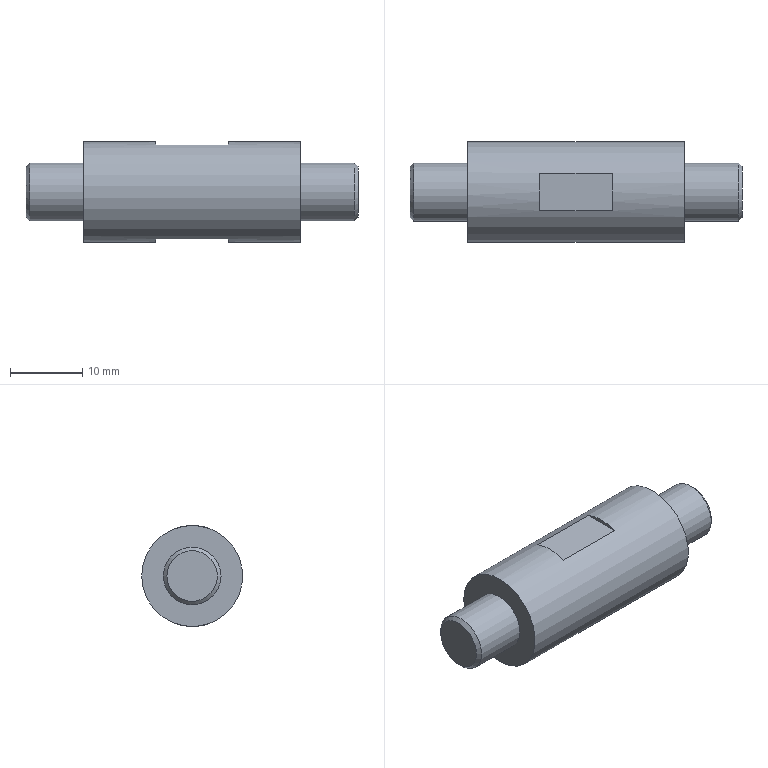Part | NX | features BREP 1 | 1 solid | 15 faces | box 46 x 14 x 14 mm | volume 5381 mm3 | plane 10 | cylinder 3 | cone 2 | commonest cylinder face diameters 8 x2 14 x1
STEP:
#1=CARTESIAN_POINT('',(-5.,-2.598,-6.5));
#2=VERTEX_POINT('',#1);
#3=CARTESIAN_POINT('',(-5.,2.598,-6.5));
#4=VERTEX_POINT('',#3);
#5=CARTESIAN_POINT('',(-5.,0.,0.));
#6=DIRECTION('',(1.,0.,0.));
#7=DIRECTION('',(0.,0.,1.));
#8=AXIS2_PLACEMENT_3D('',#5,#6,#7);
#9=CIRCLE('',#8,7.);
#10=EDGE_CURVE('',#2,#4,#9,.T.);
#11=ORIENTED_EDGE('',*,*,#10,.F.);
#12=CARTESIAN_POINT('',(5.,-2.598,-6.5));
#13=VERTEX_POINT('',#12);
#14=CARTESIAN_POINT('',(23.,-2.598,-6.5));
#15=DIRECTION('',(-1.,0.,0.));
#16=VECTOR('',#15,1000.);
#17=LINE('',#14,#16);
#18=EDGE_CURVE('',#13,#2,#17,.T.);
#19=ORIENTED_EDGE('',*,*,#18,.F.);
#20=CARTESIAN_POINT('',(5.,2.598,-6.5));
#21=VERTEX_POINT('',#20);
#22=CARTESIAN_POINT('',(5.,0.,0.));
#23=DIRECTION('',(1.,0.,0.));
#24=DIRECTION('',(0.,0.,1.));
#25=AXIS2_PLACEMENT_3D('',#22,#23,#24);
#26=CIRCLE('',#25,7.);
#27=EDGE_CURVE('',#13,#21,#26,.T.);
#28=ORIENTED_EDGE('',*,*,#27,.T.);
#29=CARTESIAN_POINT('',(23.,2.598,-6.5));
#30=DIRECTION('',(1.,0.,0.));
#31=VECTOR('',#30,1000.);
#32=LINE('',#29,#31);
#33=EDGE_CURVE('',#4,#21,#32,.T.);
#34=ORIENTED_EDGE('',*,*,#33,.F.);
#35=EDGE_LOOP('',(#11,#19,#28,#34));
#36=FACE_BOUND('',#35,.T.);
#37=CARTESIAN_POINT('',(-15.,7.,0.));
#38=VERTEX_POINT('',#37);
#39=CARTESIAN_POINT('',(-15.,0.,0.));
#40=DIRECTION('',(1.,0.,0.));
#41=DIRECTION('',(0.,1.,0.));
#42=AXIS2_PLACEMENT_3D('',#39,#40,#41);
#43=CIRCLE('',#42,7.);
#44=EDGE_CURVE('',#38,#38,#43,.T.);
#45=ORIENTED_EDGE('',*,*,#44,.T.);
#46=EDGE_LOOP('',(#45));
#47=FACE_BOUND('',#46,.T.);
#48=CARTESIAN_POINT('',(15.,7.,0.));
#49=VERTEX_POINT('',#48);
#50=CARTESIAN_POINT('',(15.,0.,0.));
#51=DIRECTION('',(1.,0.,0.));
#52=DIRECTION('',(0.,1.,0.));
#53=AXIS2_PLACEMENT_3D('',#50,#51,#52);
#54=CIRCLE('',#53,7.);
#55=EDGE_CURVE('',#49,#49,#54,.T.);
#56=ORIENTED_EDGE('',*,*,#55,.F.);
#57=EDGE_LOOP('',(#56));
#58=FACE_BOUND('',#57,.T.);
#59=CARTESIAN_POINT('',(-5.,-2.598,6.5));
#60=VERTEX_POINT('',#59);
#61=CARTESIAN_POINT('',(5.,-2.598,6.5));
#62=VERTEX_POINT('',#61);
#63=CARTESIAN_POINT('',(23.,-2.598,6.5));
#64=DIRECTION('',(1.,0.,0.));
#65=VECTOR('',#64,1000.);
#66=LINE('',#63,#65);
#67=EDGE_CURVE('',#60,#62,#66,.T.);
#68=ORIENTED_EDGE('',*,*,#67,.F.);
#69=CARTESIAN_POINT('',(-5.,2.598,6.5));
#70=VERTEX_POINT('',#69);
#71=CARTESIAN_POINT('',(-5.,0.,0.));
#72=DIRECTION('',(-1.,0.,0.));
#73=DIRECTION('',(0.,0.,-1.));
#74=AXIS2_PLACEMENT_3D('',#71,#72,#73);
#75=CIRCLE('',#74,7.);
#76=EDGE_CURVE('',#60,#70,#75,.T.);
#77=ORIENTED_EDGE('',*,*,#76,.T.);
#78=CARTESIAN_POINT('',(5.,2.598,6.5));
#79=VERTEX_POINT('',#78);
#80=CARTESIAN_POINT('',(23.,2.598,6.5));
#81=DIRECTION('',(-1.,0.,0.));
#82=VECTOR('',#81,1000.);
#83=LINE('',#80,#82);
#84=EDGE_CURVE('',#79,#70,#83,.T.);
#85=ORIENTED_EDGE('',*,*,#84,.F.);
#86=CARTESIAN_POINT('',(5.,0.,0.));
#87=DIRECTION('',(-1.,0.,0.));
#88=DIRECTION('',(0.,0.,-1.));
#89=AXIS2_PLACEMENT_3D('',#86,#87,#88);
#90=CIRCLE('',#89,7.);
#91=EDGE_CURVE('',#62,#79,#90,.T.);
#92=ORIENTED_EDGE('',*,*,#91,.F.);
#93=EDGE_LOOP('',(#68,#77,#85,#92));
#94=FACE_BOUND('',#93,.T.);
#95=CARTESIAN_POINT('',(23.,0.,0.));
#96=DIRECTION('',(1.,0.,0.));
#97=DIRECTION('',(0.,-1.,0.));
#98=AXIS2_PLACEMENT_3D('',#95,#96,#97);
#99=CYLINDRICAL_SURFACE('',#98,7.);
#100=ADVANCED_FACE('',(#36,#47,#58,#94),#99,.T.);
#101=CARTESIAN_POINT('',(23.,3.5,0.));
#102=VERTEX_POINT('',#101);
#103=CARTESIAN_POINT('',(23.,0.,0.));
#104=DIRECTION('',(1.,0.,0.));
#105=DIRECTION('',(0.,1.,0.));
#106=AXIS2_PLACEMENT_3D('',#103,#104,#105);
#107=CIRCLE('',#106,3.5);
#108=EDGE_CURVE('',#102,#102,#107,.T.);
#109=ORIENTED_EDGE('',*,*,#108,.T.);
#110=EDGE_LOOP('',(#109));
#111=FACE_BOUND('',#110,.T.);
#112=CARTESIAN_POINT('',(23.,4.,0.));
#113=DIRECTION('',(1.,0.,0.));
#114=DIRECTION('',(0.,-1.,0.));
#115=AXIS2_PLACEMENT_3D('',#112,#113,#114);
#116=PLANE('',#115);
#117=ADVANCED_FACE('',(#111),#116,.T.);
#118=CARTESIAN_POINT('',(-23.,-3.5,0.));
#119=VERTEX_POINT('',#118);
#120=CARTESIAN_POINT('',(-23.,0.,0.));
#121=DIRECTION('',(-1.,0.,0.));
#122=DIRECTION('',(0.,-1.,0.));
#123=AXIS2_PLACEMENT_3D('',#120,#121,#122);
#124=CIRCLE('',#123,3.5);
#125=EDGE_CURVE('',#119,#119,#124,.T.);
#126=ORIENTED_EDGE('',*,*,#125,.T.);
#127=EDGE_LOOP('',(#126));
#128=FACE_BOUND('',#127,.T.);
#129=CARTESIAN_POINT('',(-23.,0.,0.));
#130=DIRECTION('',(-1.,0.,0.));
#131=DIRECTION('',(0.,1.,0.));
#132=AXIS2_PLACEMENT_3D('',#129,#130,#131);
#133=PLANE('',#132);
#134=ADVANCED_FACE('',(#128),#133,.T.);
#135=CARTESIAN_POINT('',(-22.5,-4.,0.));
#136=VERTEX_POINT('',#135);
#137=CARTESIAN_POINT('',(-22.5,0.,0.));
#138=DIRECTION('',(1.,0.,0.));
#139=DIRECTION('',(0.,-1.,0.));
#140=AXIS2_PLACEMENT_3D('',#137,#138,#139);
#141=CIRCLE('',#140,4.);
#142=EDGE_CURVE('',#136,#136,#141,.T.);
#143=ORIENTED_EDGE('',*,*,#142,.T.);
#144=EDGE_LOOP('',(#143));
#145=FACE_BOUND('',#144,.T.);
#146=CARTESIAN_POINT('',(-15.,4.,0.));
#147=VERTEX_POINT('',#146);
#148=CARTESIAN_POINT('',(-15.,0.,0.));
#149=DIRECTION('',(1.,0.,0.));
#150=DIRECTION('',(0.,1.,0.));
#151=AXIS2_PLACEMENT_3D('',#148,#149,#150);
#152=CIRCLE('',#151,4.);
#153=EDGE_CURVE('',#147,#147,#152,.T.);
#154=ORIENTED_EDGE('',*,*,#153,.F.);
#155=EDGE_LOOP('',(#154));
#156=FACE_BOUND('',#155,.T.);
#157=CARTESIAN_POINT('',(23.,0.,0.));
#158=DIRECTION('',(1.,0.,0.));
#159=DIRECTION('',(0.,-1.,0.));
#160=AXIS2_PLACEMENT_3D('',#157,#158,#159);
#161=CYLINDRICAL_SURFACE('',#160,4.);
#162=ADVANCED_FACE('',(#145,#156),#161,.T.);
#163=ORIENTED_EDGE('',*,*,#153,.T.);
#164=EDGE_LOOP('',(#163));
#165=FACE_BOUND('',#164,.T.);
#166=ORIENTED_EDGE('',*,*,#44,.F.);
#167=EDGE_LOOP('',(#166));
#168=FACE_BOUND('',#167,.T.);
#169=CARTESIAN_POINT('',(-15.,4.,0.));
#170=DIRECTION('',(-1.,0.,0.));
#171=DIRECTION('',(0.,1.,0.));
#172=AXIS2_PLACEMENT_3D('',#169,#170,#171);
#173=PLANE('',#172);
#174=ADVANCED_FACE('',(#165,#168),#173,.T.);
#175=ORIENTED_EDGE('',*,*,#55,.T.);
#176=EDGE_LOOP('',(#175));
#177=FACE_BOUND('',#176,.T.);
#178=CARTESIAN_POINT('',(15.,4.,0.));
#179=VERTEX_POINT('',#178);
#180=CARTESIAN_POINT('',(15.,0.,0.));
#181=DIRECTION('',(1.,0.,0.));
#182=DIRECTION('',(0.,1.,0.));
#183=AXIS2_PLACEMENT_3D('',#180,#181,#182);
#184=CIRCLE('',#183,4.);
#185=EDGE_CURVE('',#179,#179,#184,.T.);
#186=ORIENTED_EDGE('',*,*,#185,.F.);
#187=EDGE_LOOP('',(#186));
#188=FACE_BOUND('',#187,.T.);
#189=CARTESIAN_POINT('',(15.,7.,0.));
#190=DIRECTION('',(1.,0.,0.));
#191=DIRECTION('',(0.,-1.,0.));
#192=AXIS2_PLACEMENT_3D('',#189,#190,#191);
#193=PLANE('',#192);
#194=ADVANCED_FACE('',(#177,#188),#193,.T.);
#195=CARTESIAN_POINT('',(22.5,4.,0.));
#196=VERTEX_POINT('',#195);
#197=CARTESIAN_POINT('',(22.5,0.,0.));
#198=DIRECTION('',(-1.,0.,0.));
#199=DIRECTION('',(0.,1.,0.));
#200=AXIS2_PLACEMENT_3D('',#197,#198,#199);
#201=CIRCLE('',#200,4.);
#202=EDGE_CURVE('',#196,#196,#201,.T.);
#203=ORIENTED_EDGE('',*,*,#202,.T.);
#204=EDGE_LOOP('',(#203));
#205=FACE_BOUND('',#204,.T.);
#206=ORIENTED_EDGE('',*,*,#185,.T.);
#207=EDGE_LOOP('',(#206));
#208=FACE_BOUND('',#207,.T.);
#209=CARTESIAN_POINT('',(23.,0.,0.));
#210=DIRECTION('',(1.,0.,0.));
#211=DIRECTION('',(0.,-1.,0.));
#212=AXIS2_PLACEMENT_3D('',#209,#210,#211);
#213=CYLINDRICAL_SURFACE('',#212,4.);
#214=ADVANCED_FACE('',(#205,#208),#213,.T.);
#215=ORIENTED_EDGE('',*,*,#202,.F.);
#216=EDGE_LOOP('',(#215));
#217=FACE_BOUND('',#216,.T.);
#218=ORIENTED_EDGE('',*,*,#108,.F.);
#219=EDGE_LOOP('',(#218));
#220=FACE_BOUND('',#219,.T.);
#221=CARTESIAN_POINT('',(23.,0.,0.));
#222=DIRECTION('',(-1.,0.,0.));
#223=DIRECTION('',(0.,1.,0.));
#224=AXIS2_PLACEMENT_3D('',#221,#222,#223);
#225=CONICAL_SURFACE('',#224,3.5,0.7854);
#226=ADVANCED_FACE('',(#217,#220),#225,.T.);
#227=ORIENTED_EDGE('',*,*,#125,.F.);
#228=EDGE_LOOP('',(#227));
#229=FACE_BOUND('',#228,.T.);
#230=ORIENTED_EDGE('',*,*,#142,.F.);
#231=EDGE_LOOP('',(#230));
#232=FACE_BOUND('',#231,.T.);
#233=CARTESIAN_POINT('',(-22.5,0.,0.));
#234=DIRECTION('',(1.,0.,0.));
#235=DIRECTION('',(0.,-1.,0.));
#236=AXIS2_PLACEMENT_3D('',#233,#234,#235);
#237=CONICAL_SURFACE('',#236,4.,0.7854);
#238=ADVANCED_FACE('',(#229,#232),#237,.T.);
#239=ORIENTED_EDGE('',*,*,#18,.T.);
#240=CARTESIAN_POINT('',(-5.,6.966,-6.5));
#241=DIRECTION('',(0.,-1.,0.));
#242=VECTOR('',#241,1000.);
#243=LINE('',#240,#242);
#244=EDGE_CURVE('',#4,#2,#243,.T.);
#245=ORIENTED_EDGE('',*,*,#244,.F.);
#246=ORIENTED_EDGE('',*,*,#33,.T.);
#247=CARTESIAN_POINT('',(5.,6.966,-6.5));
#248=DIRECTION('',(0.,-1.,0.));
#249=VECTOR('',#248,1000.);
#250=LINE('',#247,#249);
#251=EDGE_CURVE('',#21,#13,#250,.T.);
#252=ORIENTED_EDGE('',*,*,#251,.T.);
#253=EDGE_LOOP('',(#239,#245,#246,#252));
#254=FACE_BOUND('',#253,.T.);
#255=CARTESIAN_POINT('',(-5.,6.966,-6.5));
#256=DIRECTION('',(0.,0.,1.));
#257=DIRECTION('',(-1.,0.,0.));
#258=AXIS2_PLACEMENT_3D('',#255,#256,#257);
#259=PLANE('',#258);
#260=ADVANCED_FACE('',(#254),#259,.F.);
#261=ORIENTED_EDGE('',*,*,#10,.T.);
#262=ORIENTED_EDGE('',*,*,#244,.T.);
#263=EDGE_LOOP('',(#261,#262));
#264=FACE_BOUND('',#263,.T.);
#265=CARTESIAN_POINT('',(-5.,0.,0.));
#266=DIRECTION('',(-1.,0.,0.));
#267=DIRECTION('',(0.,0.,-1.));
#268=AXIS2_PLACEMENT_3D('',#265,#266,#267);
#269=PLANE('',#268);
#270=ADVANCED_FACE('',(#264),#269,.F.);
#271=ORIENTED_EDGE('',*,*,#251,.F.);
#272=ORIENTED_EDGE('',*,*,#27,.F.);
#273=EDGE_LOOP('',(#271,#272));
#274=FACE_BOUND('',#273,.T.);
#275=CARTESIAN_POINT('',(5.,0.,0.));
#276=DIRECTION('',(-1.,0.,0.));
#277=DIRECTION('',(0.,0.,-1.));
#278=AXIS2_PLACEMENT_3D('',#275,#276,#277);
#279=PLANE('',#278);
#280=ADVANCED_FACE('',(#274),#279,.T.);
#281=ORIENTED_EDGE('',*,*,#84,.T.);
#282=CARTESIAN_POINT('',(-5.,6.407,6.5));
#283=DIRECTION('',(0.,1.,0.));
#284=VECTOR('',#283,1000.);
#285=LINE('',#282,#284);
#286=EDGE_CURVE('',#60,#70,#285,.T.);
#287=ORIENTED_EDGE('',*,*,#286,.F.);
#288=ORIENTED_EDGE('',*,*,#67,.T.);
#289=CARTESIAN_POINT('',(5.,6.407,6.5));
#290=DIRECTION('',(0.,1.,0.));
#291=VECTOR('',#290,1000.);
#292=LINE('',#289,#291);
#293=EDGE_CURVE('',#62,#79,#292,.T.);
#294=ORIENTED_EDGE('',*,*,#293,.T.);
#295=EDGE_LOOP('',(#281,#287,#288,#294));
#296=FACE_BOUND('',#295,.T.);
#297=CARTESIAN_POINT('',(-5.,6.407,6.5));
#298=DIRECTION('',(0.,0.,-1.));
#299=DIRECTION('',(1.,0.,0.));
#300=AXIS2_PLACEMENT_3D('',#297,#298,#299);
#301=PLANE('',#300);
#302=ADVANCED_FACE('',(#296),#301,.F.);
#303=ORIENTED_EDGE('',*,*,#286,.T.);
#304=ORIENTED_EDGE('',*,*,#76,.F.);
#305=EDGE_LOOP('',(#303,#304));
#306=FACE_BOUND('',#305,.T.);
#307=CARTESIAN_POINT('',(-5.,0.,0.));
#308=DIRECTION('',(1.,0.,0.));
#309=DIRECTION('',(0.,0.,1.));
#310=AXIS2_PLACEMENT_3D('',#307,#308,#309);
#311=PLANE('',#310);
#312=ADVANCED_FACE('',(#306),#311,.T.);
#313=ORIENTED_EDGE('',*,*,#91,.T.);
#314=ORIENTED_EDGE('',*,*,#293,.F.);
#315=EDGE_LOOP('',(#313,#314));
#316=FACE_BOUND('',#315,.T.);
#317=CARTESIAN_POINT('',(5.,0.,0.));
#318=DIRECTION('',(1.,0.,0.));
#319=DIRECTION('',(0.,0.,1.));
#320=AXIS2_PLACEMENT_3D('',#317,#318,#319);
#321=PLANE('',#320);
#322=ADVANCED_FACE('',(#316),#321,.F.);
#323=CLOSED_SHELL('',(#100,#117,#134,#162,#174,#194,#214,#226,#238,#260,#270,#280,#302,#312,#322));
#324=MANIFOLD_SOLID_BREP('',#323);
#325=(LENGTH_UNIT()NAMED_UNIT(*)SI_UNIT(.MILLI.,.METRE.));
#326=UNCERTAINTY_MEASURE_WITH_UNIT(LENGTH_MEASURE(0.00001),#325,'','');
#327=(NAMED_UNIT(*)PLANE_ANGLE_UNIT()SI_UNIT($,.RADIAN.));
#328=(NAMED_UNIT(*)SI_UNIT($,.STERADIAN.)SOLID_ANGLE_UNIT());
#329=(GEOMETRIC_REPRESENTATION_CONTEXT(3)GLOBAL_UNCERTAINTY_ASSIGNED_CONTEXT((#326))GLOBAL_UNIT_ASSIGNED_CONTEXT((#325,#327,#328))REPRESENTATION_CONTEXT('',''));
#330=ADVANCED_BREP_SHAPE_REPRESENTATION('',(#324),#329);